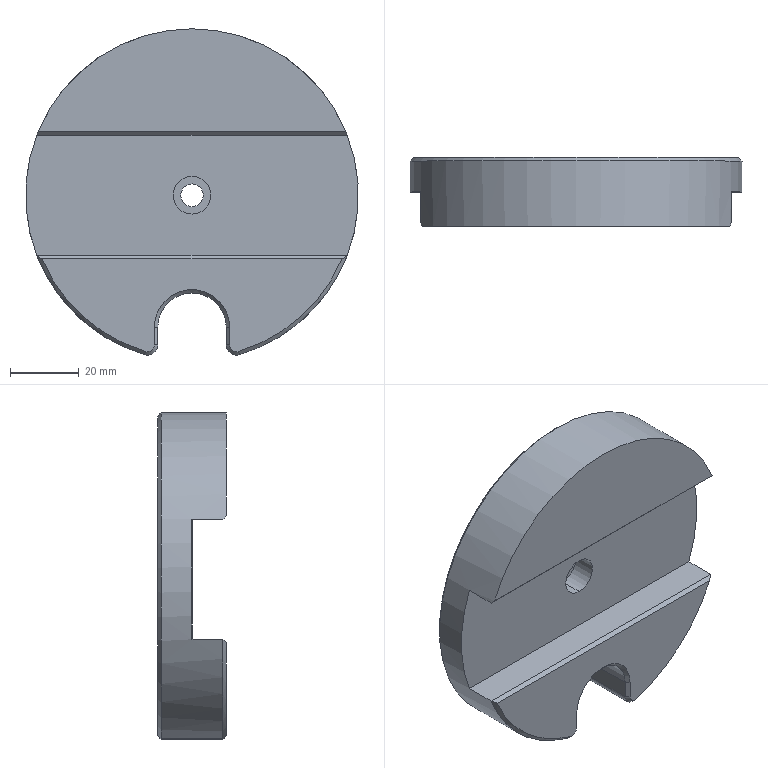Part | STEP file | PN_0012 Counterweight block | 1 solid | 37 faces | box 97 x 20 x 95.103 mm | volume 106377 mm3 | plane 15 | cone 11 | cylinder 11 | commonest cylinder face diameters 6 x4 6.6 x2 11 x2 20 x2 97 x1